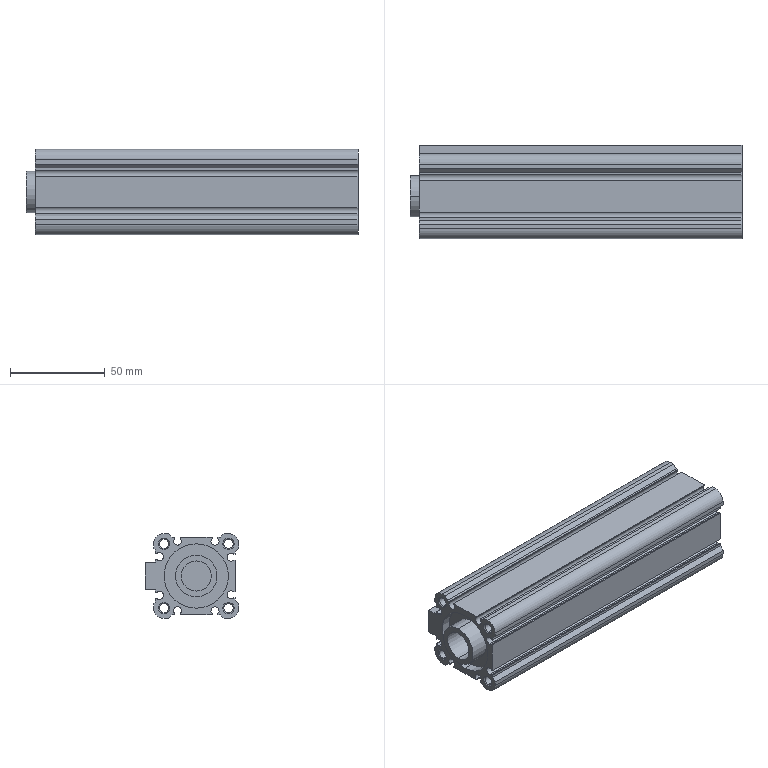Part | STEP file | 1 | 1 solid | 145 faces | box 175.5 x 49.5 x 45 mm | volume 171932 mm3 | plane 65 | cylinder 60 | cone 20 | commonest cylinder face diameters 4.26 x18 4.917 x16 6 x8 8.566 x4 11 x4 34 x4